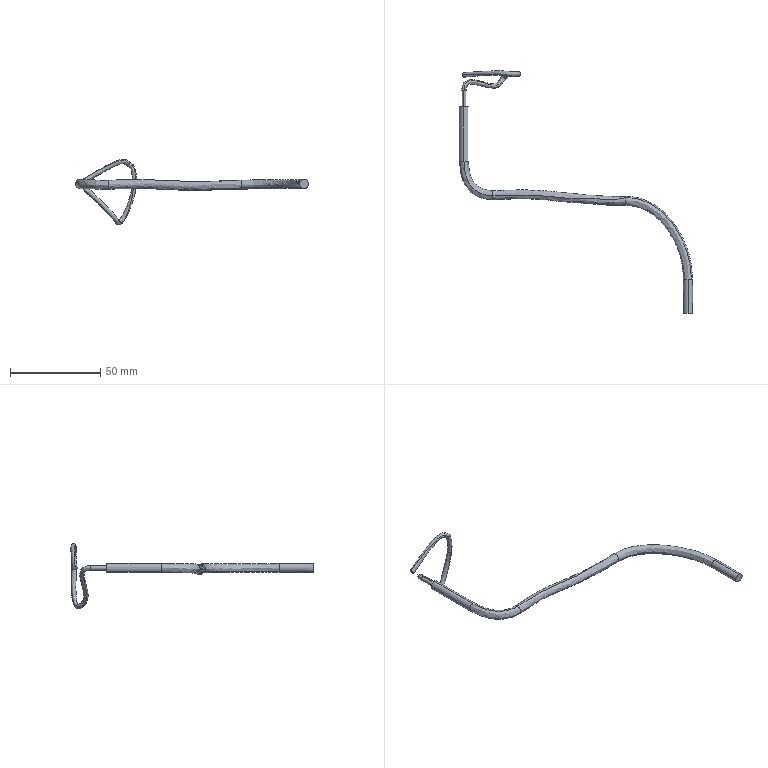Part | SolidWorks | features 3DProfileFeature 4, Sweep 2 | 1 solid | 19 faces | box 128.902 x 134.039 x 36.156 mm | volume 4687 mm3 | spline 10 | cylinder 6 | plane 3 | commonest cylinder face diameters 5 x4 2.5 x2